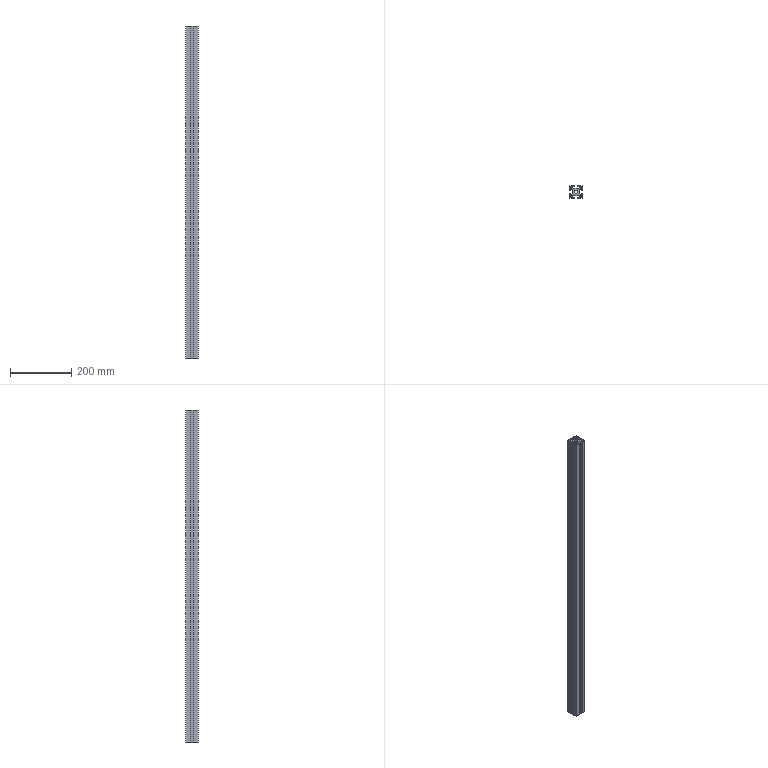Part | SolidWorks | features BaseBody 1 | 1 solid | 56 faces | box 40 x 40 x 1080 mm | volume 860018 mm3 | plane 46 | cylinder 10 | commonest cylinder face diameters 6 x8 10.5 x2